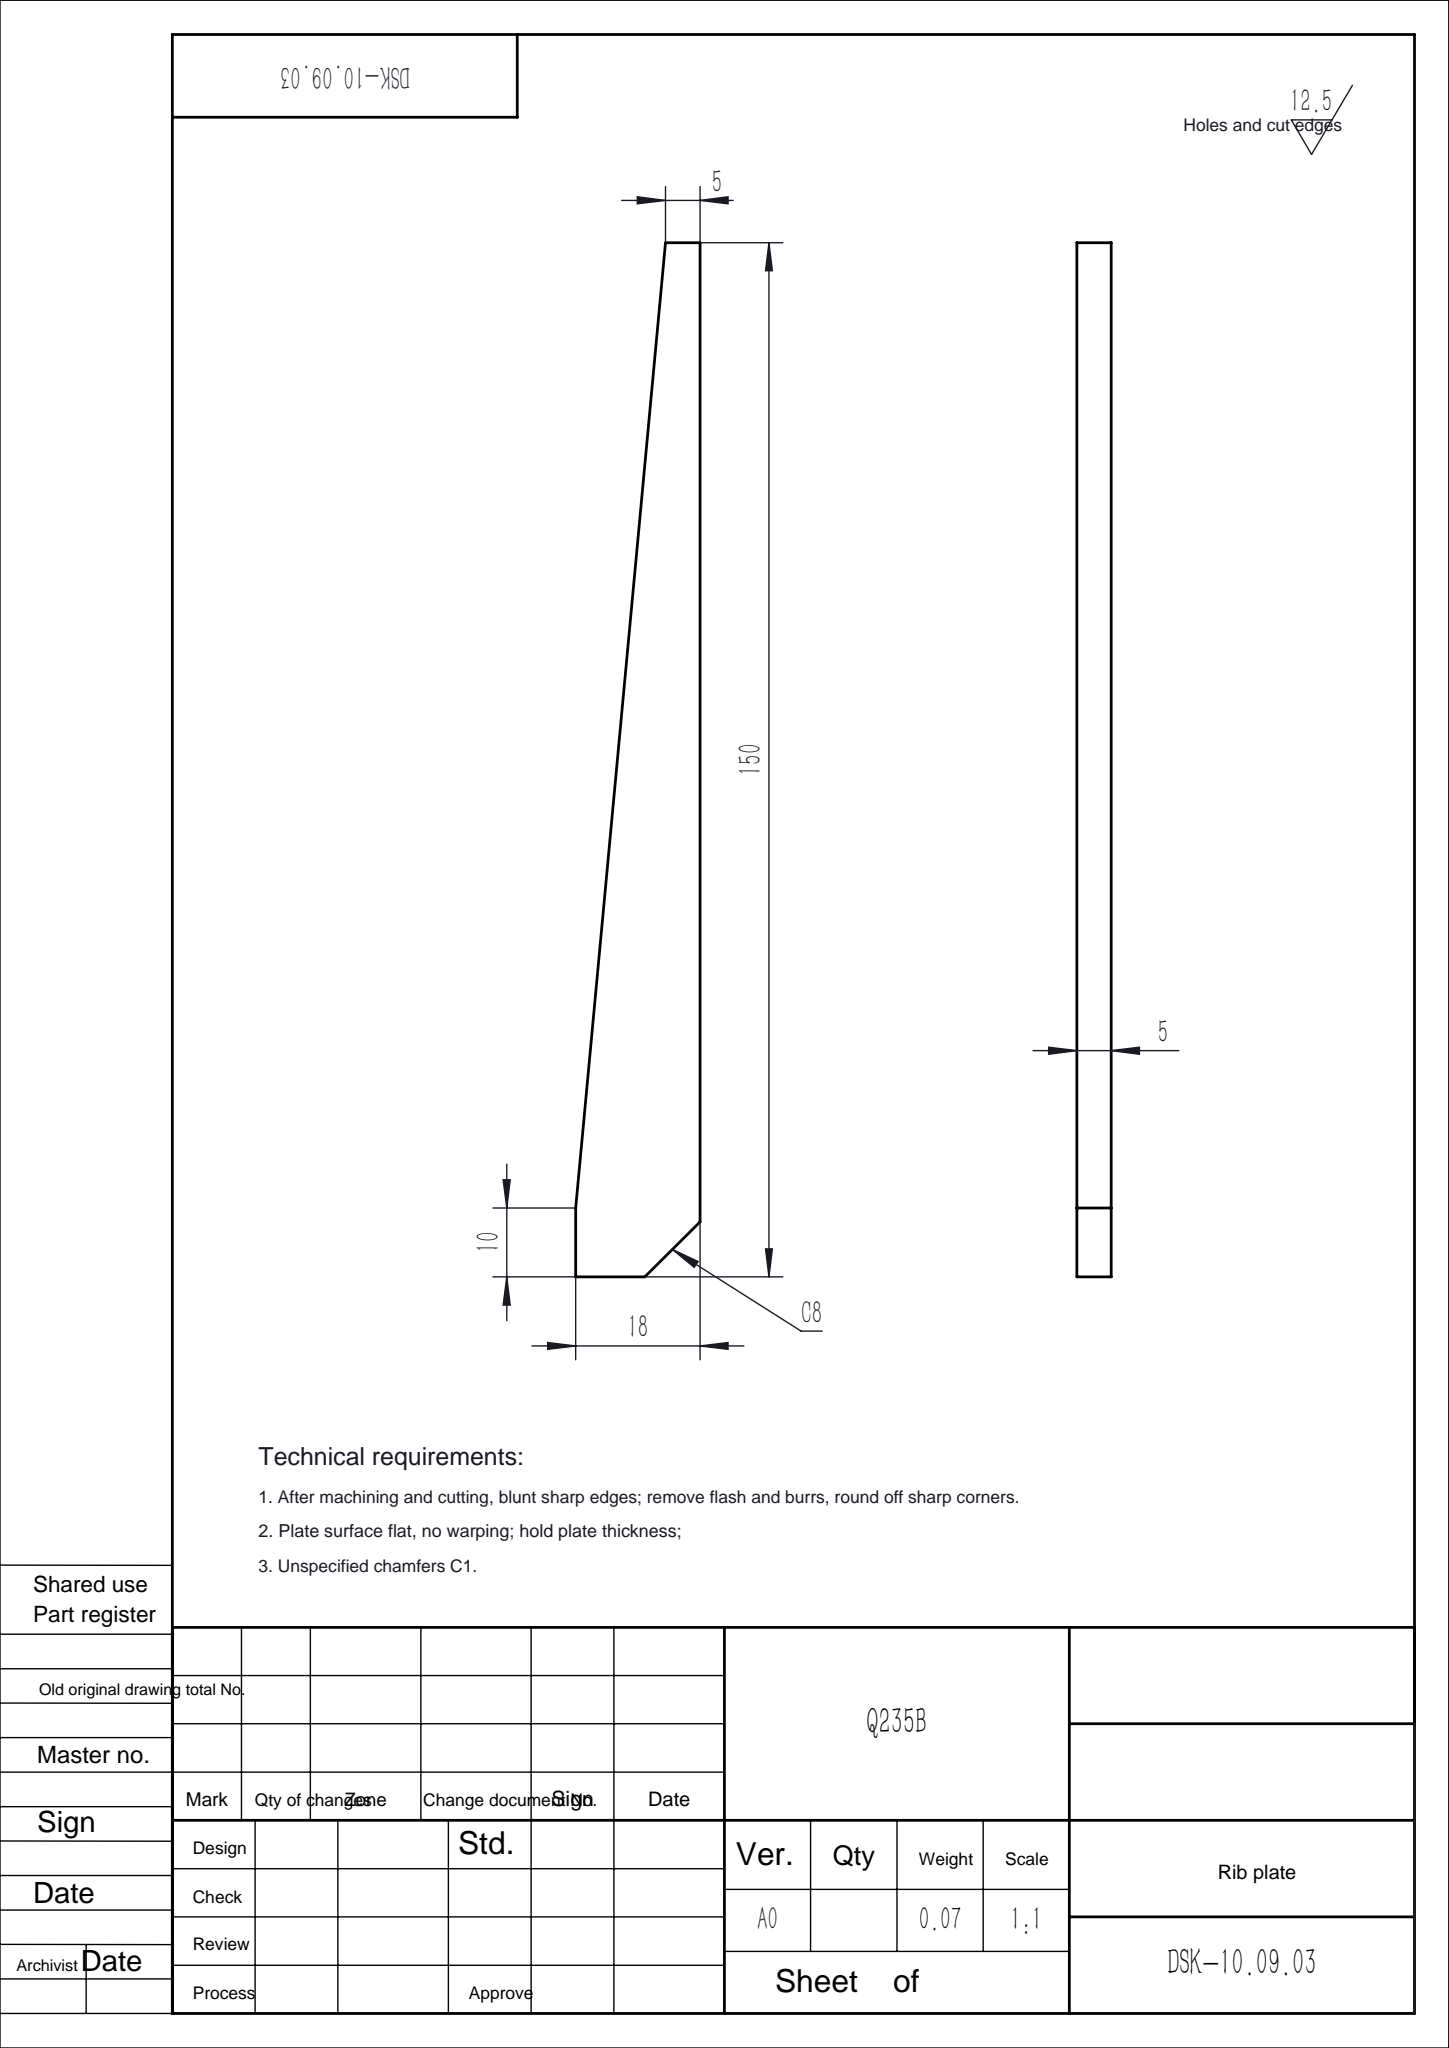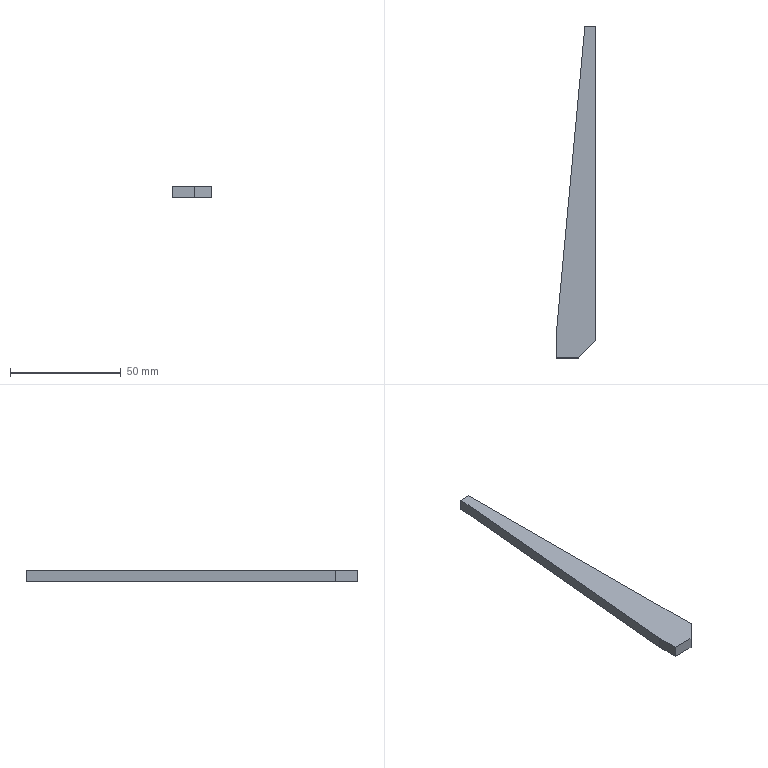Part | SolidWorks | features Extrusion 1 | 1 solid | 8 faces | box 18 x 150 x 5 mm | volume 8790 mm3 | plane 8
STEP:
#1=CARTESIAN_POINT('',(0.,0.,0.));
#2=VERTEX_POINT('',#1);
#3=CARTESIAN_POINT('',(10.,0.,0.));
#4=VERTEX_POINT('',#3);
#5=CARTESIAN_POINT('',(10.,0.,0.));
#6=DIRECTION('',(1.,0.,0.));
#7=VECTOR('',#6,1000.);
#8=LINE('',#5,#7);
#9=EDGE_CURVE('',#2,#4,#8,.T.);
#10=ORIENTED_EDGE('',*,*,#9,.T.);
#11=CARTESIAN_POINT('',(10.,0.,5.));
#12=VERTEX_POINT('',#11);
#13=CARTESIAN_POINT('',(10.,0.,5.));
#14=DIRECTION('',(0.,0.,-1.));
#15=VECTOR('',#14,1000.);
#16=LINE('',#13,#15);
#17=EDGE_CURVE('',#12,#4,#16,.T.);
#18=ORIENTED_EDGE('',*,*,#17,.F.);
#19=CARTESIAN_POINT('',(0.,0.,5.));
#20=VERTEX_POINT('',#19);
#21=CARTESIAN_POINT('',(10.,0.,5.));
#22=DIRECTION('',(1.,0.,0.));
#23=VECTOR('',#22,1000.);
#24=LINE('',#21,#23);
#25=EDGE_CURVE('',#20,#12,#24,.T.);
#26=ORIENTED_EDGE('',*,*,#25,.F.);
#27=CARTESIAN_POINT('',(0.,0.,5.));
#28=DIRECTION('',(0.,0.,-1.));
#29=VECTOR('',#28,1000.);
#30=LINE('',#27,#29);
#31=EDGE_CURVE('',#20,#2,#30,.T.);
#32=ORIENTED_EDGE('',*,*,#31,.T.);
#33=EDGE_LOOP('',(#10,#18,#26,#32));
#34=FACE_OUTER_BOUND('',#33,.T.);
#35=CARTESIAN_POINT('',(10.,0.,5.));
#36=DIRECTION('',(0.,1.,0.));
#37=DIRECTION('',(-1.,0.,0.));
#38=AXIS2_PLACEMENT_3D('',#35,#36,#37);
#39=PLANE('',#38);
#40=ADVANCED_FACE('',(#34),#39,.F.);
#41=CARTESIAN_POINT('',(18.,8.,0.));
#42=VERTEX_POINT('',#41);
#43=CARTESIAN_POINT('',(18.,8.,0.));
#44=DIRECTION('',(0.7071,0.7071,0.));
#45=VECTOR('',#44,1000.);
#46=LINE('',#43,#45);
#47=EDGE_CURVE('',#4,#42,#46,.T.);
#48=ORIENTED_EDGE('',*,*,#47,.T.);
#49=CARTESIAN_POINT('',(18.,8.,5.));
#50=VERTEX_POINT('',#49);
#51=CARTESIAN_POINT('',(18.,8.,5.));
#52=DIRECTION('',(0.,0.,-1.));
#53=VECTOR('',#52,1000.);
#54=LINE('',#51,#53);
#55=EDGE_CURVE('',#50,#42,#54,.T.);
#56=ORIENTED_EDGE('',*,*,#55,.F.);
#57=CARTESIAN_POINT('',(18.,8.,5.));
#58=DIRECTION('',(0.7071,0.7071,0.));
#59=VECTOR('',#58,1000.);
#60=LINE('',#57,#59);
#61=EDGE_CURVE('',#12,#50,#60,.T.);
#62=ORIENTED_EDGE('',*,*,#61,.F.);
#63=ORIENTED_EDGE('',*,*,#17,.T.);
#64=EDGE_LOOP('',(#48,#56,#62,#63));
#65=FACE_OUTER_BOUND('',#64,.T.);
#66=CARTESIAN_POINT('',(18.,8.,5.));
#67=DIRECTION('',(-0.7071,0.7071,0.));
#68=DIRECTION('',(-0.7071,-0.7071,0.));
#69=AXIS2_PLACEMENT_3D('',#66,#67,#68);
#70=PLANE('',#69);
#71=ADVANCED_FACE('',(#65),#70,.F.);
#72=CARTESIAN_POINT('',(18.,150.,0.));
#73=VERTEX_POINT('',#72);
#74=CARTESIAN_POINT('',(18.,150.,0.));
#75=DIRECTION('',(0.,1.,0.));
#76=VECTOR('',#75,1000.);
#77=LINE('',#74,#76);
#78=EDGE_CURVE('',#42,#73,#77,.T.);
#79=ORIENTED_EDGE('',*,*,#78,.T.);
#80=CARTESIAN_POINT('',(18.,150.,5.));
#81=VERTEX_POINT('',#80);
#82=CARTESIAN_POINT('',(18.,150.,5.));
#83=DIRECTION('',(0.,0.,-1.));
#84=VECTOR('',#83,1000.);
#85=LINE('',#82,#84);
#86=EDGE_CURVE('',#81,#73,#85,.T.);
#87=ORIENTED_EDGE('',*,*,#86,.F.);
#88=CARTESIAN_POINT('',(18.,150.,5.));
#89=DIRECTION('',(0.,1.,0.));
#90=VECTOR('',#89,1000.);
#91=LINE('',#88,#90);
#92=EDGE_CURVE('',#50,#81,#91,.T.);
#93=ORIENTED_EDGE('',*,*,#92,.F.);
#94=ORIENTED_EDGE('',*,*,#55,.T.);
#95=EDGE_LOOP('',(#79,#87,#93,#94));
#96=FACE_OUTER_BOUND('',#95,.T.);
#97=CARTESIAN_POINT('',(18.,150.,5.));
#98=DIRECTION('',(-1.,0.,0.));
#99=DIRECTION('',(0.,-1.,0.));
#100=AXIS2_PLACEMENT_3D('',#97,#98,#99);
#101=PLANE('',#100);
#102=ADVANCED_FACE('',(#96),#101,.F.);
#103=CARTESIAN_POINT('',(13.,150.,0.));
#104=VERTEX_POINT('',#103);
#105=CARTESIAN_POINT('',(13.,150.,0.));
#106=DIRECTION('',(-1.,0.,0.));
#107=VECTOR('',#106,1000.);
#108=LINE('',#105,#107);
#109=EDGE_CURVE('',#73,#104,#108,.T.);
#110=ORIENTED_EDGE('',*,*,#109,.T.);
#111=CARTESIAN_POINT('',(13.,150.,5.));
#112=VERTEX_POINT('',#111);
#113=CARTESIAN_POINT('',(13.,150.,5.));
#114=DIRECTION('',(0.,0.,-1.));
#115=VECTOR('',#114,1000.);
#116=LINE('',#113,#115);
#117=EDGE_CURVE('',#112,#104,#116,.T.);
#118=ORIENTED_EDGE('',*,*,#117,.F.);
#119=CARTESIAN_POINT('',(13.,150.,5.));
#120=DIRECTION('',(-1.,0.,0.));
#121=VECTOR('',#120,1000.);
#122=LINE('',#119,#121);
#123=EDGE_CURVE('',#81,#112,#122,.T.);
#124=ORIENTED_EDGE('',*,*,#123,.F.);
#125=ORIENTED_EDGE('',*,*,#86,.T.);
#126=EDGE_LOOP('',(#110,#118,#124,#125));
#127=FACE_OUTER_BOUND('',#126,.T.);
#128=CARTESIAN_POINT('',(13.,150.,5.));
#129=DIRECTION('',(0.,-1.,0.));
#130=DIRECTION('',(0.,0.,-1.));
#131=AXIS2_PLACEMENT_3D('',#128,#129,#130);
#132=PLANE('',#131);
#133=ADVANCED_FACE('',(#127),#132,.F.);
#134=CARTESIAN_POINT('',(0.,10.,0.));
#135=VERTEX_POINT('',#134);
#136=CARTESIAN_POINT('',(0.,10.,0.));
#137=DIRECTION('',(-0.09246,-0.9957,0.));
#138=VECTOR('',#137,1000.);
#139=LINE('',#136,#138);
#140=EDGE_CURVE('',#104,#135,#139,.T.);
#141=ORIENTED_EDGE('',*,*,#140,.T.);
#142=CARTESIAN_POINT('',(0.,10.,5.));
#143=VERTEX_POINT('',#142);
#144=CARTESIAN_POINT('',(0.,10.,5.));
#145=DIRECTION('',(0.,0.,-1.));
#146=VECTOR('',#145,1000.);
#147=LINE('',#144,#146);
#148=EDGE_CURVE('',#143,#135,#147,.T.);
#149=ORIENTED_EDGE('',*,*,#148,.F.);
#150=CARTESIAN_POINT('',(0.,10.,5.));
#151=DIRECTION('',(-0.09246,-0.9957,0.));
#152=VECTOR('',#151,1000.);
#153=LINE('',#150,#152);
#154=EDGE_CURVE('',#112,#143,#153,.T.);
#155=ORIENTED_EDGE('',*,*,#154,.F.);
#156=ORIENTED_EDGE('',*,*,#117,.T.);
#157=EDGE_LOOP('',(#141,#149,#155,#156));
#158=FACE_OUTER_BOUND('',#157,.T.);
#159=CARTESIAN_POINT('',(0.,10.,5.));
#160=DIRECTION('',(0.9957,-0.09246,0.));
#161=DIRECTION('',(0.09246,0.9957,0.));
#162=AXIS2_PLACEMENT_3D('',#159,#160,#161);
#163=PLANE('',#162);
#164=ADVANCED_FACE('',(#158),#163,.F.);
#165=CARTESIAN_POINT('',(0.,0.,0.));
#166=DIRECTION('',(0.,-1.,0.));
#167=VECTOR('',#166,1000.);
#168=LINE('',#165,#167);
#169=EDGE_CURVE('',#135,#2,#168,.T.);
#170=ORIENTED_EDGE('',*,*,#169,.T.);
#171=ORIENTED_EDGE('',*,*,#31,.F.);
#172=CARTESIAN_POINT('',(0.,0.,5.));
#173=DIRECTION('',(0.,-1.,0.));
#174=VECTOR('',#173,1000.);
#175=LINE('',#172,#174);
#176=EDGE_CURVE('',#143,#20,#175,.T.);
#177=ORIENTED_EDGE('',*,*,#176,.F.);
#178=ORIENTED_EDGE('',*,*,#148,.T.);
#179=EDGE_LOOP('',(#170,#171,#177,#178));
#180=FACE_OUTER_BOUND('',#179,.T.);
#181=CARTESIAN_POINT('',(0.,0.,5.));
#182=DIRECTION('',(1.,0.,0.));
#183=DIRECTION('',(0.,0.,-1.));
#184=AXIS2_PLACEMENT_3D('',#181,#182,#183);
#185=PLANE('',#184);
#186=ADVANCED_FACE('',(#180),#185,.F.);
#187=ORIENTED_EDGE('',*,*,#25,.T.);
#188=ORIENTED_EDGE('',*,*,#61,.T.);
#189=ORIENTED_EDGE('',*,*,#92,.T.);
#190=ORIENTED_EDGE('',*,*,#123,.T.);
#191=ORIENTED_EDGE('',*,*,#154,.T.);
#192=ORIENTED_EDGE('',*,*,#176,.T.);
#193=EDGE_LOOP('',(#187,#188,#189,#190,#191,#192));
#194=FACE_OUTER_BOUND('',#193,.T.);
#195=CARTESIAN_POINT('',(0.,0.,5.));
#196=DIRECTION('',(0.,0.,-1.));
#197=DIRECTION('',(-1.,0.,0.));
#198=AXIS2_PLACEMENT_3D('',#195,#196,#197);
#199=PLANE('',#198);
#200=ADVANCED_FACE('',(#194),#199,.F.);
#201=ORIENTED_EDGE('',*,*,#9,.F.);
#202=ORIENTED_EDGE('',*,*,#169,.F.);
#203=ORIENTED_EDGE('',*,*,#140,.F.);
#204=ORIENTED_EDGE('',*,*,#109,.F.);
#205=ORIENTED_EDGE('',*,*,#78,.F.);
#206=ORIENTED_EDGE('',*,*,#47,.F.);
#207=EDGE_LOOP('',(#201,#202,#203,#204,#205,#206));
#208=FACE_OUTER_BOUND('',#207,.T.);
#209=CARTESIAN_POINT('',(0.,0.,0.));
#210=DIRECTION('',(0.,0.,-1.));
#211=DIRECTION('',(-1.,0.,0.));
#212=AXIS2_PLACEMENT_3D('',#209,#210,#211);
#213=PLANE('',#212);
#214=ADVANCED_FACE('',(#208),#213,.T.);
#215=CLOSED_SHELL('',(#40,#71,#102,#133,#164,#186,#200,#214));
#216=MANIFOLD_SOLID_BREP('',#215);
#217=CARTESIAN_POINT('',(0.,0.,0.));
#218=DIRECTION('',(0.,0.,1.));
#219=DIRECTION('',(1.,0.,0.));
#220=AXIS2_PLACEMENT_3D('',#217,#218,#219);
#221=(LENGTH_UNIT()NAMED_UNIT(*)SI_UNIT(.MILLI.,.METRE.));
#222=UNCERTAINTY_MEASURE_WITH_UNIT(LENGTH_MEASURE(0.00001),#221,'','');
#223=(NAMED_UNIT(*)PLANE_ANGLE_UNIT()SI_UNIT($,.RADIAN.));
#224=(NAMED_UNIT(*)SI_UNIT($,.STERADIAN.)SOLID_ANGLE_UNIT());
#225=(GEOMETRIC_REPRESENTATION_CONTEXT(3)GLOBAL_UNCERTAINTY_ASSIGNED_CONTEXT((#222))GLOBAL_UNIT_ASSIGNED_CONTEXT((#221,#223,#224))REPRESENTATION_CONTEXT('',''));
#226=ADVANCED_BREP_SHAPE_REPRESENTATION('',(#216,#220),#225);